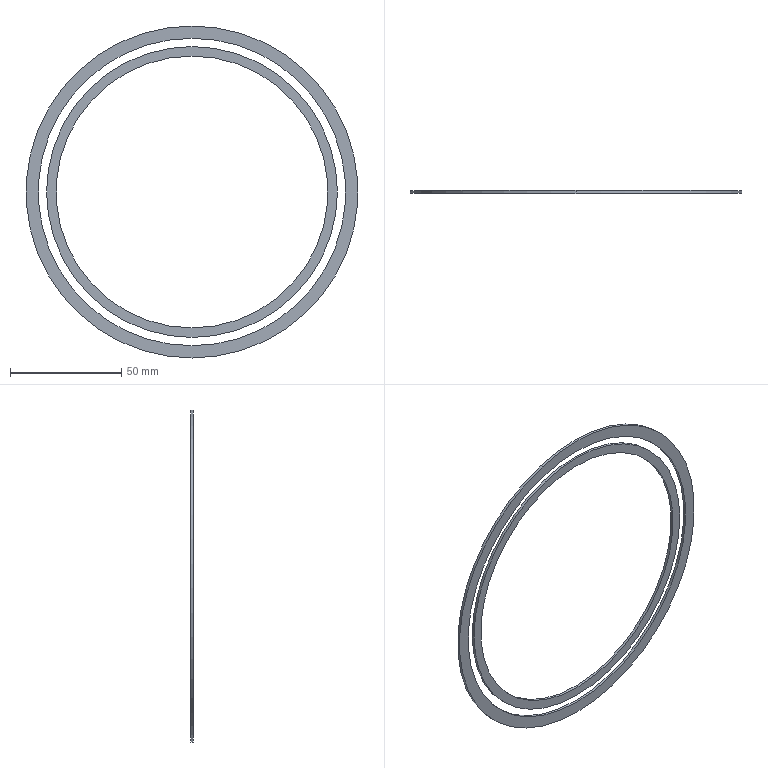Part | SolidWorks | features Revolution 1 | 2 solids | 12 faces | box 148.991 x 1.185 x 148.991 mm | volume 4958 mm3 | cylinder 8 | plane 4 | commonest cylinder face diameters 121.991 x2 130.524 x2 137.942 x2 148.991 x2
STEP:
#1=CARTESIAN_POINT('',(0.,136.315,-68.971));
#2=VERTEX_POINT('',#1);
#3=CARTESIAN_POINT('',(0.,136.315,68.971));
#4=VERTEX_POINT('',#3);
#5=CARTESIAN_POINT('',(0.,136.315,0.));
#6=DIRECTION('',(0.,1.,0.));
#7=DIRECTION('',(0.,0.,1.));
#8=AXIS2_PLACEMENT_3D('',#5,#6,#7);
#9=CIRCLE('',#8,68.971);
#10=EDGE_CURVE('',#2,#4,#9,.T.);
#11=ORIENTED_EDGE('',*,*,#10,.F.);
#12=CARTESIAN_POINT('',(0.,137.5,-68.971));
#13=VERTEX_POINT('',#12);
#14=CARTESIAN_POINT('',(0.,0.,-68.971));
#15=DIRECTION('',(0.,1.,0.));
#16=VECTOR('',#15,1000.);
#17=LINE('',#14,#16);
#18=EDGE_CURVE('',#2,#13,#17,.T.);
#19=ORIENTED_EDGE('',*,*,#18,.T.);
#20=CARTESIAN_POINT('',(0.,137.5,68.971));
#21=VERTEX_POINT('',#20);
#22=CARTESIAN_POINT('',(0.,137.5,0.));
#23=DIRECTION('',(0.,1.,0.));
#24=DIRECTION('',(0.,0.,1.));
#25=AXIS2_PLACEMENT_3D('',#22,#23,#24);
#26=CIRCLE('',#25,68.971);
#27=EDGE_CURVE('',#13,#21,#26,.T.);
#28=ORIENTED_EDGE('',*,*,#27,.T.);
#29=CARTESIAN_POINT('',(0.,0.,68.971));
#30=DIRECTION('',(0.,1.,0.));
#31=VECTOR('',#30,1000.);
#32=LINE('',#29,#31);
#33=EDGE_CURVE('',#4,#21,#32,.T.);
#34=ORIENTED_EDGE('',*,*,#33,.F.);
#35=EDGE_LOOP('',(#11,#19,#28,#34));
#36=FACE_OUTER_BOUND('',#35,.T.);
#37=CARTESIAN_POINT('',(0.,0.,0.));
#38=DIRECTION('',(0.,1.,0.));
#39=DIRECTION('',(0.,0.,1.));
#40=AXIS2_PLACEMENT_3D('',#37,#38,#39);
#41=CYLINDRICAL_SURFACE('',#40,68.971);
#42=ADVANCED_FACE('',(#36),#41,.F.);
#43=CARTESIAN_POINT('',(0.,136.315,74.496));
#44=VERTEX_POINT('',#43);
#45=CARTESIAN_POINT('',(0.,136.315,-74.496));
#46=VERTEX_POINT('',#45);
#47=CARTESIAN_POINT('',(0.,136.315,0.));
#48=DIRECTION('',(0.,1.,0.));
#49=DIRECTION('',(0.,0.,1.));
#50=AXIS2_PLACEMENT_3D('',#47,#48,#49);
#51=CIRCLE('',#50,74.496);
#52=EDGE_CURVE('',#44,#46,#51,.T.);
#53=ORIENTED_EDGE('',*,*,#52,.T.);
#54=CARTESIAN_POINT('',(0.,137.5,-74.496));
#55=VERTEX_POINT('',#54);
#56=CARTESIAN_POINT('',(0.,0.,-74.496));
#57=DIRECTION('',(0.,1.,0.));
#58=VECTOR('',#57,1000.);
#59=LINE('',#56,#58);
#60=EDGE_CURVE('',#46,#55,#59,.T.);
#61=ORIENTED_EDGE('',*,*,#60,.T.);
#62=CARTESIAN_POINT('',(0.,137.5,74.496));
#63=VERTEX_POINT('',#62);
#64=CARTESIAN_POINT('',(0.,137.5,0.));
#65=DIRECTION('',(0.,1.,0.));
#66=DIRECTION('',(0.,0.,1.));
#67=AXIS2_PLACEMENT_3D('',#64,#65,#66);
#68=CIRCLE('',#67,74.496);
#69=EDGE_CURVE('',#63,#55,#68,.T.);
#70=ORIENTED_EDGE('',*,*,#69,.F.);
#71=CARTESIAN_POINT('',(0.,0.,74.496));
#72=DIRECTION('',(0.,1.,0.));
#73=VECTOR('',#72,1000.);
#74=LINE('',#71,#73);
#75=EDGE_CURVE('',#44,#63,#74,.T.);
#76=ORIENTED_EDGE('',*,*,#75,.F.);
#77=EDGE_LOOP('',(#53,#61,#70,#76));
#78=FACE_OUTER_BOUND('',#77,.T.);
#79=CARTESIAN_POINT('',(0.,0.,0.));
#80=DIRECTION('',(0.,1.,0.));
#81=DIRECTION('',(0.,0.,1.));
#82=AXIS2_PLACEMENT_3D('',#79,#80,#81);
#83=CYLINDRICAL_SURFACE('',#82,74.496);
#84=ADVANCED_FACE('',(#78),#83,.T.);
#85=ORIENTED_EDGE('',*,*,#60,.F.);
#86=CARTESIAN_POINT('',(0.,136.315,0.));
#87=DIRECTION('',(0.,1.,0.));
#88=DIRECTION('',(0.,0.,1.));
#89=AXIS2_PLACEMENT_3D('',#86,#87,#88);
#90=CIRCLE('',#89,74.496);
#91=EDGE_CURVE('',#46,#44,#90,.T.);
#92=ORIENTED_EDGE('',*,*,#91,.T.);
#93=ORIENTED_EDGE('',*,*,#75,.T.);
#94=CARTESIAN_POINT('',(0.,137.5,0.));
#95=DIRECTION('',(0.,1.,0.));
#96=DIRECTION('',(0.,0.,1.));
#97=AXIS2_PLACEMENT_3D('',#94,#95,#96);
#98=CIRCLE('',#97,74.496);
#99=EDGE_CURVE('',#55,#63,#98,.T.);
#100=ORIENTED_EDGE('',*,*,#99,.F.);
#101=EDGE_LOOP('',(#85,#92,#93,#100));
#102=FACE_OUTER_BOUND('',#101,.T.);
#103=CARTESIAN_POINT('',(0.,0.,0.));
#104=DIRECTION('',(0.,1.,0.));
#105=DIRECTION('',(0.,0.,1.));
#106=AXIS2_PLACEMENT_3D('',#103,#104,#105);
#107=CYLINDRICAL_SURFACE('',#106,74.496);
#108=ADVANCED_FACE('',(#102),#107,.T.);
#109=ORIENTED_EDGE('',*,*,#52,.F.);
#110=ORIENTED_EDGE('',*,*,#91,.F.);
#111=EDGE_LOOP('',(#109,#110));
#112=FACE_OUTER_BOUND('',#111,.T.);
#113=CARTESIAN_POINT('',(0.,136.315,0.));
#114=DIRECTION('',(0.,1.,0.));
#115=DIRECTION('',(0.,0.,1.));
#116=AXIS2_PLACEMENT_3D('',#113,#114,#115);
#117=CIRCLE('',#116,68.971);
#118=EDGE_CURVE('',#4,#2,#117,.T.);
#119=ORIENTED_EDGE('',*,*,#118,.T.);
#120=ORIENTED_EDGE('',*,*,#10,.T.);
#121=EDGE_LOOP('',(#119,#120));
#122=FACE_BOUND('',#121,.T.);
#123=CARTESIAN_POINT('',(74.496,136.315,0.));
#124=DIRECTION('',(0.,1.,0.));
#125=DIRECTION('',(0.,0.,1.));
#126=AXIS2_PLACEMENT_3D('',#123,#124,#125);
#127=PLANE('',#126);
#128=ADVANCED_FACE('',(#112,#122),#127,.F.);
#129=ORIENTED_EDGE('',*,*,#18,.F.);
#130=ORIENTED_EDGE('',*,*,#118,.F.);
#131=ORIENTED_EDGE('',*,*,#33,.T.);
#132=CARTESIAN_POINT('',(0.,137.5,0.));
#133=DIRECTION('',(0.,1.,0.));
#134=DIRECTION('',(0.,0.,1.));
#135=AXIS2_PLACEMENT_3D('',#132,#133,#134);
#136=CIRCLE('',#135,68.971);
#137=EDGE_CURVE('',#21,#13,#136,.T.);
#138=ORIENTED_EDGE('',*,*,#137,.T.);
#139=EDGE_LOOP('',(#129,#130,#131,#138));
#140=FACE_OUTER_BOUND('',#139,.T.);
#141=CARTESIAN_POINT('',(0.,0.,0.));
#142=DIRECTION('',(0.,1.,0.));
#143=DIRECTION('',(0.,0.,1.));
#144=AXIS2_PLACEMENT_3D('',#141,#142,#143);
#145=CYLINDRICAL_SURFACE('',#144,68.971);
#146=ADVANCED_FACE('',(#140),#145,.F.);
#147=ORIENTED_EDGE('',*,*,#137,.F.);
#148=ORIENTED_EDGE('',*,*,#27,.F.);
#149=EDGE_LOOP('',(#147,#148));
#150=FACE_BOUND('',#149,.T.);
#151=ORIENTED_EDGE('',*,*,#69,.T.);
#152=ORIENTED_EDGE('',*,*,#99,.T.);
#153=EDGE_LOOP('',(#151,#152));
#154=FACE_OUTER_BOUND('',#153,.T.);
#155=CARTESIAN_POINT('',(74.496,137.5,0.));
#156=DIRECTION('',(0.,-1.,0.));
#157=DIRECTION('',(0.,0.,-1.));
#158=AXIS2_PLACEMENT_3D('',#155,#156,#157);
#159=PLANE('',#158);
#160=ADVANCED_FACE('',(#150,#154),#159,.F.);
#161=CLOSED_SHELL('',(#42,#84,#108,#128,#146,#160));
#162=MANIFOLD_SOLID_BREP('',#161);
#163=CARTESIAN_POINT('',(0.,136.315,65.262));
#164=VERTEX_POINT('',#163);
#165=CARTESIAN_POINT('',(0.,136.315,-65.262));
#166=VERTEX_POINT('',#165);
#167=CARTESIAN_POINT('',(0.,136.315,0.));
#168=DIRECTION('',(0.,1.,0.));
#169=DIRECTION('',(0.,0.,1.));
#170=AXIS2_PLACEMENT_3D('',#167,#168,#169);
#171=CIRCLE('',#170,65.262);
#172=EDGE_CURVE('',#164,#166,#171,.T.);
#173=ORIENTED_EDGE('',*,*,#172,.T.);
#174=CARTESIAN_POINT('',(0.,137.5,-65.262));
#175=VERTEX_POINT('',#174);
#176=CARTESIAN_POINT('',(0.,0.,-65.262));
#177=DIRECTION('',(0.,1.,0.));
#178=VECTOR('',#177,1000.);
#179=LINE('',#176,#178);
#180=EDGE_CURVE('',#166,#175,#179,.T.);
#181=ORIENTED_EDGE('',*,*,#180,.T.);
#182=CARTESIAN_POINT('',(0.,137.5,65.262));
#183=VERTEX_POINT('',#182);
#184=CARTESIAN_POINT('',(0.,137.5,0.));
#185=DIRECTION('',(0.,1.,0.));
#186=DIRECTION('',(0.,0.,1.));
#187=AXIS2_PLACEMENT_3D('',#184,#185,#186);
#188=CIRCLE('',#187,65.262);
#189=EDGE_CURVE('',#183,#175,#188,.T.);
#190=ORIENTED_EDGE('',*,*,#189,.F.);
#191=CARTESIAN_POINT('',(0.,0.,65.262));
#192=DIRECTION('',(0.,1.,0.));
#193=VECTOR('',#192,1000.);
#194=LINE('',#191,#193);
#195=EDGE_CURVE('',#164,#183,#194,.T.);
#196=ORIENTED_EDGE('',*,*,#195,.F.);
#197=EDGE_LOOP('',(#173,#181,#190,#196));
#198=FACE_OUTER_BOUND('',#197,.T.);
#199=CARTESIAN_POINT('',(0.,0.,0.));
#200=DIRECTION('',(0.,1.,0.));
#201=DIRECTION('',(0.,0.,1.));
#202=AXIS2_PLACEMENT_3D('',#199,#200,#201);
#203=CYLINDRICAL_SURFACE('',#202,65.262);
#204=ADVANCED_FACE('',(#198),#203,.T.);
#205=CARTESIAN_POINT('',(0.,136.315,-60.996));
#206=VERTEX_POINT('',#205);
#207=CARTESIAN_POINT('',(0.,136.315,60.996));
#208=VERTEX_POINT('',#207);
#209=CARTESIAN_POINT('',(0.,136.315,0.));
#210=DIRECTION('',(0.,1.,0.));
#211=DIRECTION('',(0.,0.,1.));
#212=AXIS2_PLACEMENT_3D('',#209,#210,#211);
#213=CIRCLE('',#212,60.996);
#214=EDGE_CURVE('',#206,#208,#213,.T.);
#215=ORIENTED_EDGE('',*,*,#214,.F.);
#216=CARTESIAN_POINT('',(0.,137.5,-60.996));
#217=VERTEX_POINT('',#216);
#218=CARTESIAN_POINT('',(0.,0.,-60.996));
#219=DIRECTION('',(0.,1.,0.));
#220=VECTOR('',#219,1000.);
#221=LINE('',#218,#220);
#222=EDGE_CURVE('',#206,#217,#221,.T.);
#223=ORIENTED_EDGE('',*,*,#222,.T.);
#224=CARTESIAN_POINT('',(0.,137.5,60.996));
#225=VERTEX_POINT('',#224);
#226=CARTESIAN_POINT('',(0.,137.5,0.));
#227=DIRECTION('',(0.,1.,0.));
#228=DIRECTION('',(0.,0.,1.));
#229=AXIS2_PLACEMENT_3D('',#226,#227,#228);
#230=CIRCLE('',#229,60.996);
#231=EDGE_CURVE('',#217,#225,#230,.T.);
#232=ORIENTED_EDGE('',*,*,#231,.T.);
#233=CARTESIAN_POINT('',(0.,0.,60.996));
#234=DIRECTION('',(0.,1.,0.));
#235=VECTOR('',#234,1000.);
#236=LINE('',#233,#235);
#237=EDGE_CURVE('',#208,#225,#236,.T.);
#238=ORIENTED_EDGE('',*,*,#237,.F.);
#239=EDGE_LOOP('',(#215,#223,#232,#238));
#240=FACE_OUTER_BOUND('',#239,.T.);
#241=CARTESIAN_POINT('',(0.,0.,0.));
#242=DIRECTION('',(0.,1.,0.));
#243=DIRECTION('',(0.,0.,1.));
#244=AXIS2_PLACEMENT_3D('',#241,#242,#243);
#245=CYLINDRICAL_SURFACE('',#244,60.996);
#246=ADVANCED_FACE('',(#240),#245,.F.);
#247=ORIENTED_EDGE('',*,*,#222,.F.);
#248=CARTESIAN_POINT('',(0.,136.315,0.));
#249=DIRECTION('',(0.,1.,0.));
#250=DIRECTION('',(0.,0.,1.));
#251=AXIS2_PLACEMENT_3D('',#248,#249,#250);
#252=CIRCLE('',#251,60.996);
#253=EDGE_CURVE('',#208,#206,#252,.T.);
#254=ORIENTED_EDGE('',*,*,#253,.F.);
#255=ORIENTED_EDGE('',*,*,#237,.T.);
#256=CARTESIAN_POINT('',(0.,137.5,0.));
#257=DIRECTION('',(0.,1.,0.));
#258=DIRECTION('',(0.,0.,1.));
#259=AXIS2_PLACEMENT_3D('',#256,#257,#258);
#260=CIRCLE('',#259,60.996);
#261=EDGE_CURVE('',#225,#217,#260,.T.);
#262=ORIENTED_EDGE('',*,*,#261,.T.);
#263=EDGE_LOOP('',(#247,#254,#255,#262));
#264=FACE_OUTER_BOUND('',#263,.T.);
#265=CARTESIAN_POINT('',(0.,0.,0.));
#266=DIRECTION('',(0.,1.,0.));
#267=DIRECTION('',(0.,0.,1.));
#268=AXIS2_PLACEMENT_3D('',#265,#266,#267);
#269=CYLINDRICAL_SURFACE('',#268,60.996);
#270=ADVANCED_FACE('',(#264),#269,.F.);
#271=ORIENTED_EDGE('',*,*,#172,.F.);
#272=CARTESIAN_POINT('',(0.,136.315,0.));
#273=DIRECTION('',(0.,1.,0.));
#274=DIRECTION('',(0.,0.,1.));
#275=AXIS2_PLACEMENT_3D('',#272,#273,#274);
#276=CIRCLE('',#275,65.262);
#277=EDGE_CURVE('',#166,#164,#276,.T.);
#278=ORIENTED_EDGE('',*,*,#277,.F.);
#279=EDGE_LOOP('',(#271,#278));
#280=FACE_OUTER_BOUND('',#279,.T.);
#281=ORIENTED_EDGE('',*,*,#253,.T.);
#282=ORIENTED_EDGE('',*,*,#214,.T.);
#283=EDGE_LOOP('',(#281,#282));
#284=FACE_BOUND('',#283,.T.);
#285=CARTESIAN_POINT('',(60.996,136.315,0.));
#286=DIRECTION('',(0.,1.,0.));
#287=DIRECTION('',(0.,0.,1.));
#288=AXIS2_PLACEMENT_3D('',#285,#286,#287);
#289=PLANE('',#288);
#290=ADVANCED_FACE('',(#280,#284),#289,.F.);
#291=ORIENTED_EDGE('',*,*,#180,.F.);
#292=ORIENTED_EDGE('',*,*,#277,.T.);
#293=ORIENTED_EDGE('',*,*,#195,.T.);
#294=CARTESIAN_POINT('',(0.,137.5,0.));
#295=DIRECTION('',(0.,1.,0.));
#296=DIRECTION('',(0.,0.,1.));
#297=AXIS2_PLACEMENT_3D('',#294,#295,#296);
#298=CIRCLE('',#297,65.262);
#299=EDGE_CURVE('',#175,#183,#298,.T.);
#300=ORIENTED_EDGE('',*,*,#299,.F.);
#301=EDGE_LOOP('',(#291,#292,#293,#300));
#302=FACE_OUTER_BOUND('',#301,.T.);
#303=CARTESIAN_POINT('',(0.,0.,0.));
#304=DIRECTION('',(0.,1.,0.));
#305=DIRECTION('',(0.,0.,1.));
#306=AXIS2_PLACEMENT_3D('',#303,#304,#305);
#307=CYLINDRICAL_SURFACE('',#306,65.262);
#308=ADVANCED_FACE('',(#302),#307,.T.);
#309=ORIENTED_EDGE('',*,*,#261,.F.);
#310=ORIENTED_EDGE('',*,*,#231,.F.);
#311=EDGE_LOOP('',(#309,#310));
#312=FACE_BOUND('',#311,.T.);
#313=ORIENTED_EDGE('',*,*,#189,.T.);
#314=ORIENTED_EDGE('',*,*,#299,.T.);
#315=EDGE_LOOP('',(#313,#314));
#316=FACE_OUTER_BOUND('',#315,.T.);
#317=CARTESIAN_POINT('',(60.996,137.5,0.));
#318=DIRECTION('',(0.,-1.,0.));
#319=DIRECTION('',(0.,0.,-1.));
#320=AXIS2_PLACEMENT_3D('',#317,#318,#319);
#321=PLANE('',#320);
#322=ADVANCED_FACE('',(#312,#316),#321,.F.);
#323=CLOSED_SHELL('',(#204,#246,#270,#290,#308,#322));
#324=MANIFOLD_SOLID_BREP('',#323);
#325=CARTESIAN_POINT('',(0.,0.,0.));
#326=DIRECTION('',(0.,0.,1.));
#327=DIRECTION('',(1.,0.,0.));
#328=AXIS2_PLACEMENT_3D('',#325,#326,#327);
#329=(LENGTH_UNIT()NAMED_UNIT(*)SI_UNIT(.MILLI.,.METRE.));
#330=UNCERTAINTY_MEASURE_WITH_UNIT(LENGTH_MEASURE(0.00001),#329,'','');
#331=(NAMED_UNIT(*)PLANE_ANGLE_UNIT()SI_UNIT($,.RADIAN.));
#332=(NAMED_UNIT(*)SI_UNIT($,.STERADIAN.)SOLID_ANGLE_UNIT());
#333=(GEOMETRIC_REPRESENTATION_CONTEXT(3)GLOBAL_UNCERTAINTY_ASSIGNED_CONTEXT((#330))GLOBAL_UNIT_ASSIGNED_CONTEXT((#329,#331,#332))REPRESENTATION_CONTEXT('',''));
#334=ADVANCED_BREP_SHAPE_REPRESENTATION('',(#162,#324,#328),#333);